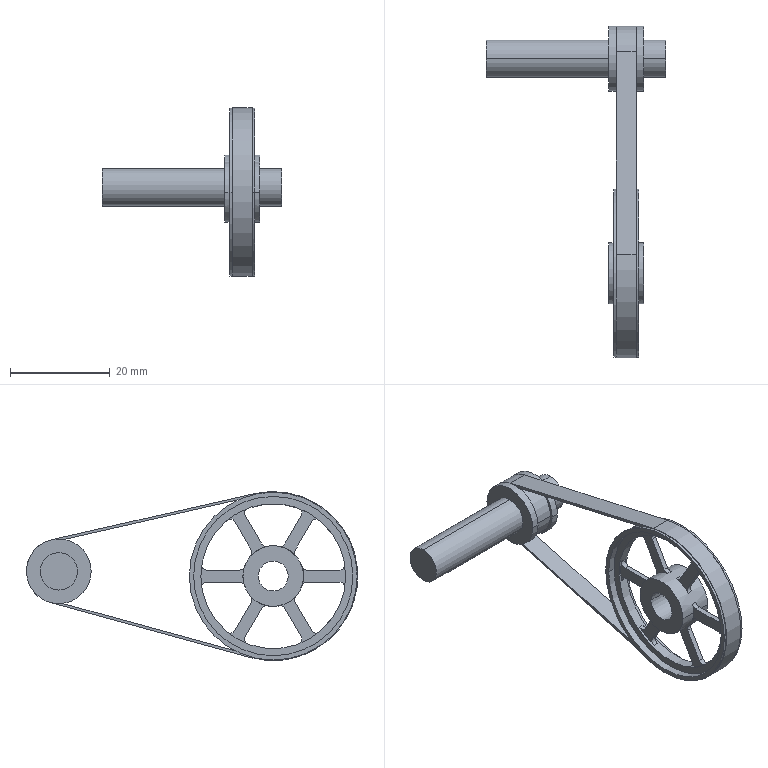Part | SolidWorks | features ICE 6, Cut 2, Fillet 2, Extrusion 1 | 3 solids | 106 faces | box 36 x 66.386 x 33.884 mm | volume 3751 mm3 | cylinder 62 | plane 44 | commonest cylinder face diameters 2 x30 12.984 x6 7.484 x4 11.996 x4 31.895 x4 33.613 x4